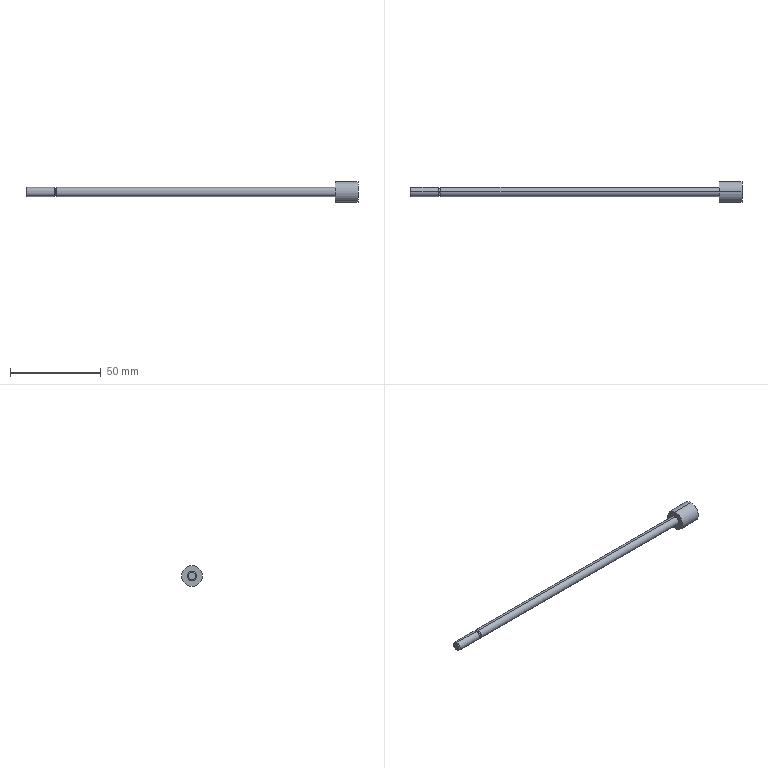Part | STEP file | 001-004-12PB125URod | 1 solid | 16 faces | box 182.85 x 11.5 x 11.5 mm | volume 4627 mm3 | cylinder 8 | cone 4 | plane 4 | commonest cylinder face diameters 5 x4 4.38 x2 11.5 x2
STEP:
#1=CARTESIAN_POINT('',(0.,0.,0.));
#2=DIRECTION('',(0.,0.,1.));
#3=DIRECTION('',(1.,0.,0.));
#4=AXIS2_PLACEMENT_3D('',#1,#2,#3);
#5=CARTESIAN_POINT('',(182.85,0.,5.75));
#6=VERTEX_POINT('',#5);
#7=CARTESIAN_POINT('',(182.85,0.,-5.75));
#8=VERTEX_POINT('',#7);
#9=CARTESIAN_POINT('',(182.85,0.,0.));
#10=DIRECTION('',(-1.,0.,0.));
#11=DIRECTION('',(0.,0.,1.));
#12=AXIS2_PLACEMENT_3D('',#9,#10,#11);
#13=CIRCLE('',#12,5.75);
#14=CARTESIAN_POINT('',(182.85,0.,0.));
#15=DIRECTION('',(-1.,0.,0.));
#16=DIRECTION('',(0.,0.,1.));
#17=AXIS2_PLACEMENT_3D('',#14,#15,#16);
#18=CYLINDRICAL_SURFACE('',#17,5.75);
#19=CARTESIAN_POINT('',(0.,0.));
#20=DIRECTION('',(1.,0.));
#21=VECTOR('',#20,1.);
#22=LINE('',#19,#21);
#23=(GEOMETRIC_REPRESENTATION_CONTEXT(2)PARAMETRIC_REPRESENTATION_CONTEXT()REPRESENTATION_CONTEXT('',''));
#24=DEFINITIONAL_REPRESENTATION('',(#22),#23);
#25=PCURVE('',#18,#24);
#26=CARTESIAN_POINT('',(182.85,5.75,0.));
#27=DIRECTION('',(-1.,0.,0.));
#28=DIRECTION('',(0.,0.,1.));
#29=AXIS2_PLACEMENT_3D('',#26,#27,#28);
#30=PLANE('',#29);
#31=CARTESIAN_POINT('',(0.,-5.75));
#32=DIRECTION('',(1.,0.));
#33=AXIS2_PLACEMENT_2D('',#31,#32);
#34=CIRCLE('',#33,5.75);
#35=(GEOMETRIC_REPRESENTATION_CONTEXT(2)PARAMETRIC_REPRESENTATION_CONTEXT()REPRESENTATION_CONTEXT('',''));
#36=DEFINITIONAL_REPRESENTATION('',(#34),#35);
#37=PCURVE('',#30,#36);
#38=SURFACE_CURVE('',#13,(#25,#37),.PCURVE_S1.);
#39=EDGE_CURVE('',#6,#8,#38,.T.);
#40=ORIENTED_EDGE('',*,*,#39,.T.);
#41=CARTESIAN_POINT('',(170.45,0.,-5.75));
#42=VERTEX_POINT('',#41);
#43=CARTESIAN_POINT('',(182.85,0.,-5.75));
#44=DIRECTION('',(-1.,0.,0.));
#45=VECTOR('',#44,1.);
#46=LINE('',#43,#45);
#47=CARTESIAN_POINT('',(3.142,0.));
#48=DIRECTION('',(0.,1.));
#49=VECTOR('',#48,1.);
#50=LINE('',#47,#49);
#51=(GEOMETRIC_REPRESENTATION_CONTEXT(2)PARAMETRIC_REPRESENTATION_CONTEXT()REPRESENTATION_CONTEXT('',''));
#52=DEFINITIONAL_REPRESENTATION('',(#50),#51);
#53=PCURVE('',#18,#52);
#54=CARTESIAN_POINT('',(182.85,0.,0.));
#55=DIRECTION('',(-1.,0.,0.));
#56=DIRECTION('',(0.,0.,1.));
#57=AXIS2_PLACEMENT_3D('',#54,#55,#56);
#58=CYLINDRICAL_SURFACE('',#57,5.75);
#59=CARTESIAN_POINT('',(3.142,0.));
#60=DIRECTION('',(0.,1.));
#61=VECTOR('',#60,1.);
#62=LINE('',#59,#61);
#63=(GEOMETRIC_REPRESENTATION_CONTEXT(2)PARAMETRIC_REPRESENTATION_CONTEXT()REPRESENTATION_CONTEXT('',''));
#64=DEFINITIONAL_REPRESENTATION('',(#62),#63);
#65=PCURVE('',#58,#64);
#66=SURFACE_CURVE('',#46,(#53,#65),.PCURVE_S1.);
#67=EDGE_CURVE('',#8,#42,#66,.T.);
#68=ORIENTED_EDGE('',*,*,#67,.T.);
#69=CARTESIAN_POINT('',(170.45,0.,5.75));
#70=VERTEX_POINT('',#69);
#71=CARTESIAN_POINT('',(170.45,0.,0.));
#72=DIRECTION('',(-1.,0.,0.));
#73=DIRECTION('',(0.,0.,1.));
#74=AXIS2_PLACEMENT_3D('',#71,#72,#73);
#75=CIRCLE('',#74,5.75);
#76=CARTESIAN_POINT('',(0.,12.4));
#77=DIRECTION('',(1.,0.));
#78=VECTOR('',#77,1.);
#79=LINE('',#76,#78);
#80=(GEOMETRIC_REPRESENTATION_CONTEXT(2)PARAMETRIC_REPRESENTATION_CONTEXT()REPRESENTATION_CONTEXT('',''));
#81=DEFINITIONAL_REPRESENTATION('',(#79),#80);
#82=PCURVE('',#18,#81);
#83=CARTESIAN_POINT('',(170.45,2.5,0.));
#84=DIRECTION('',(1.,0.,0.));
#85=DIRECTION('',(0.,0.,-1.));
#86=AXIS2_PLACEMENT_3D('',#83,#84,#85);
#87=PLANE('',#86);
#88=CARTESIAN_POINT('',(-5.75,-2.5));
#89=CARTESIAN_POINT('',(-5.75,7.459));
#90=CARTESIAN_POINT('',(2.875,2.48));
#91=CARTESIAN_POINT('',(11.5,-2.5));
#92=CARTESIAN_POINT('',(2.875,-7.48));
#93=CARTESIAN_POINT('',(-5.75,-12.459));
#94=CARTESIAN_POINT('',(-5.75,-2.5));
#95=(BOUNDED_CURVE()B_SPLINE_CURVE(2,(#88,#89,#90,#91,#92,#93,#94),.UNSPECIFIED.,.T.,.F.)B_SPLINE_CURVE_WITH_KNOTS((1,2,2,2,2,1),(-2.094,0.,2.094,4.189,6.283,8.378),.UNSPECIFIED.)CURVE()GEOMETRIC_REPRESENTATION_ITEM()RATIONAL_B_SPLINE_CURVE((1.,0.5,1.,0.5,1.,0.5,1.))REPRESENTATION_ITEM(''));
#96=(GEOMETRIC_REPRESENTATION_CONTEXT(2)PARAMETRIC_REPRESENTATION_CONTEXT()REPRESENTATION_CONTEXT('',''));
#97=DEFINITIONAL_REPRESENTATION('',(#95),#96);
#98=PCURVE('',#87,#97);
#99=SURFACE_CURVE('',#75,(#82,#98),.PCURVE_S1.);
#100=EDGE_CURVE('',#70,#42,#99,.T.);
#101=ORIENTED_EDGE('',*,*,#100,.F.);
#102=CARTESIAN_POINT('',(182.85,0.,5.75));
#103=DIRECTION('',(-1.,0.,0.));
#104=VECTOR('',#103,1.);
#105=LINE('',#102,#104);
#106=CARTESIAN_POINT('',(0.,0.));
#107=DIRECTION('',(0.,1.));
#108=VECTOR('',#107,1.);
#109=LINE('',#106,#108);
#110=(GEOMETRIC_REPRESENTATION_CONTEXT(2)PARAMETRIC_REPRESENTATION_CONTEXT()REPRESENTATION_CONTEXT('',''));
#111=DEFINITIONAL_REPRESENTATION('',(#109),#110);
#112=PCURVE('',#18,#111);
#113=CARTESIAN_POINT('',(6.283,0.));
#114=DIRECTION('',(0.,1.));
#115=VECTOR('',#114,1.);
#116=LINE('',#113,#115);
#117=(GEOMETRIC_REPRESENTATION_CONTEXT(2)PARAMETRIC_REPRESENTATION_CONTEXT()REPRESENTATION_CONTEXT('',''));
#118=DEFINITIONAL_REPRESENTATION('',(#116),#117);
#119=PCURVE('',#58,#118);
#120=SURFACE_CURVE('',#105,(#112,#119),.PCURVE_S1.);
#121=EDGE_CURVE('',#6,#70,#120,.T.);
#122=ORIENTED_EDGE('',*,*,#121,.F.);
#123=EDGE_LOOP('',(#40,#68,#101,#122));
#124=FACE_BOUND('',#123,.T.);
#125=ADVANCED_FACE('',(#124),#18,.T.);
#126=CARTESIAN_POINT('',(170.45,0.,2.5));
#127=VERTEX_POINT('',#126);
#128=CARTESIAN_POINT('',(170.45,0.,-2.5));
#129=VERTEX_POINT('',#128);
#130=CARTESIAN_POINT('',(170.45,0.,0.));
#131=DIRECTION('',(-1.,0.,0.));
#132=DIRECTION('',(0.,0.,1.));
#133=AXIS2_PLACEMENT_3D('',#130,#131,#132);
#134=CIRCLE('',#133,2.5);
#135=CARTESIAN_POINT('',(182.85,0.,0.));
#136=DIRECTION('',(-1.,0.,0.));
#137=DIRECTION('',(0.,0.,1.));
#138=AXIS2_PLACEMENT_3D('',#135,#136,#137);
#139=CYLINDRICAL_SURFACE('',#138,2.5);
#140=CARTESIAN_POINT('',(0.,12.4));
#141=DIRECTION('',(1.,0.));
#142=VECTOR('',#141,1.);
#143=LINE('',#140,#142);
#144=(GEOMETRIC_REPRESENTATION_CONTEXT(2)PARAMETRIC_REPRESENTATION_CONTEXT()REPRESENTATION_CONTEXT('',''));
#145=DEFINITIONAL_REPRESENTATION('',(#143),#144);
#146=PCURVE('',#139,#145);
#147=CARTESIAN_POINT('',(-2.5,-2.5));
#148=CARTESIAN_POINT('',(-2.5,1.83));
#149=CARTESIAN_POINT('',(1.25,-0.3349));
#150=CARTESIAN_POINT('',(5.,-2.5));
#151=CARTESIAN_POINT('',(1.25,-4.665));
#152=CARTESIAN_POINT('',(-2.5,-6.83));
#153=CARTESIAN_POINT('',(-2.5,-2.5));
#154=(BOUNDED_CURVE()B_SPLINE_CURVE(2,(#147,#148,#149,#150,#151,#152,#153),.UNSPECIFIED.,.T.,.F.)B_SPLINE_CURVE_WITH_KNOTS((1,2,2,2,2,1),(-2.094,0.,2.094,4.189,6.283,8.378),.UNSPECIFIED.)CURVE()GEOMETRIC_REPRESENTATION_ITEM()RATIONAL_B_SPLINE_CURVE((1.,0.5,1.,0.5,1.,0.5,1.))REPRESENTATION_ITEM(''));
#155=(GEOMETRIC_REPRESENTATION_CONTEXT(2)PARAMETRIC_REPRESENTATION_CONTEXT()REPRESENTATION_CONTEXT('',''));
#156=DEFINITIONAL_REPRESENTATION('',(#154),#155);
#157=PCURVE('',#87,#156);
#158=SURFACE_CURVE('',#134,(#146,#157),.PCURVE_S1.);
#159=EDGE_CURVE('',#127,#129,#158,.T.);
#160=ORIENTED_EDGE('',*,*,#159,.T.);
#161=CARTESIAN_POINT('',(17.,0.,-2.5));
#162=VERTEX_POINT('',#161);
#163=CARTESIAN_POINT('',(182.85,0.,-2.5));
#164=DIRECTION('',(-1.,0.,0.));
#165=VECTOR('',#164,1.);
#166=LINE('',#163,#165);
#167=CARTESIAN_POINT('',(3.142,0.));
#168=DIRECTION('',(0.,1.));
#169=VECTOR('',#168,1.);
#170=LINE('',#167,#169);
#171=(GEOMETRIC_REPRESENTATION_CONTEXT(2)PARAMETRIC_REPRESENTATION_CONTEXT()REPRESENTATION_CONTEXT('',''));
#172=DEFINITIONAL_REPRESENTATION('',(#170),#171);
#173=PCURVE('',#139,#172);
#174=CARTESIAN_POINT('',(182.85,0.,0.));
#175=DIRECTION('',(-1.,0.,0.));
#176=DIRECTION('',(0.,0.,1.));
#177=AXIS2_PLACEMENT_3D('',#174,#175,#176);
#178=CYLINDRICAL_SURFACE('',#177,2.5);
#179=CARTESIAN_POINT('',(3.142,0.));
#180=DIRECTION('',(0.,1.));
#181=VECTOR('',#180,1.);
#182=LINE('',#179,#181);
#183=(GEOMETRIC_REPRESENTATION_CONTEXT(2)PARAMETRIC_REPRESENTATION_CONTEXT()REPRESENTATION_CONTEXT('',''));
#184=DEFINITIONAL_REPRESENTATION('',(#182),#183);
#185=PCURVE('',#178,#184);
#186=SURFACE_CURVE('',#166,(#173,#185),.PCURVE_S1.);
#187=EDGE_CURVE('',#129,#162,#186,.T.);
#188=ORIENTED_EDGE('',*,*,#187,.T.);
#189=CARTESIAN_POINT('',(17.,0.,2.5));
#190=VERTEX_POINT('',#189);
#191=CARTESIAN_POINT('',(17.,0.,0.));
#192=DIRECTION('',(-1.,0.,0.));
#193=DIRECTION('',(0.,0.,1.));
#194=AXIS2_PLACEMENT_3D('',#191,#192,#193);
#195=CIRCLE('',#194,2.5);
#196=CARTESIAN_POINT('',(0.,165.85));
#197=DIRECTION('',(1.,0.));
#198=VECTOR('',#197,1.);
#199=LINE('',#196,#198);
#200=(GEOMETRIC_REPRESENTATION_CONTEXT(2)PARAMETRIC_REPRESENTATION_CONTEXT()REPRESENTATION_CONTEXT('',''));
#201=DEFINITIONAL_REPRESENTATION('',(#199),#200);
#202=PCURVE('',#139,#201);
#203=CARTESIAN_POINT('',(17.,0.,0.));
#204=DIRECTION('',(1.,0.,0.));
#205=DIRECTION('',(0.,0.,-1.));
#206=AXIS2_PLACEMENT_3D('',#203,#204,#205);
#207=CONICAL_SURFACE('',#206,2.5,0.555);
#208=CARTESIAN_POINT('',(3.142,0.));
#209=DIRECTION('',(-1.,0.));
#210=VECTOR('',#209,1.);
#211=LINE('',#208,#210);
#212=(GEOMETRIC_REPRESENTATION_CONTEXT(2)PARAMETRIC_REPRESENTATION_CONTEXT()REPRESENTATION_CONTEXT('',''));
#213=DEFINITIONAL_REPRESENTATION('',(#211),#212);
#214=PCURVE('',#207,#213);
#215=SURFACE_CURVE('',#195,(#202,#214),.PCURVE_S1.);
#216=EDGE_CURVE('',#190,#162,#215,.T.);
#217=ORIENTED_EDGE('',*,*,#216,.F.);
#218=CARTESIAN_POINT('',(182.85,0.,2.5));
#219=DIRECTION('',(-1.,0.,0.));
#220=VECTOR('',#219,1.);
#221=LINE('',#218,#220);
#222=CARTESIAN_POINT('',(0.,0.));
#223=DIRECTION('',(0.,1.));
#224=VECTOR('',#223,1.);
#225=LINE('',#222,#224);
#226=(GEOMETRIC_REPRESENTATION_CONTEXT(2)PARAMETRIC_REPRESENTATION_CONTEXT()REPRESENTATION_CONTEXT('',''));
#227=DEFINITIONAL_REPRESENTATION('',(#225),#226);
#228=PCURVE('',#139,#227);
#229=CARTESIAN_POINT('',(6.283,0.));
#230=DIRECTION('',(0.,1.));
#231=VECTOR('',#230,1.);
#232=LINE('',#229,#231);
#233=(GEOMETRIC_REPRESENTATION_CONTEXT(2)PARAMETRIC_REPRESENTATION_CONTEXT()REPRESENTATION_CONTEXT('',''));
#234=DEFINITIONAL_REPRESENTATION('',(#232),#233);
#235=PCURVE('',#178,#234);
#236=SURFACE_CURVE('',#221,(#228,#235),.PCURVE_S1.);
#237=EDGE_CURVE('',#127,#190,#236,.T.);
#238=ORIENTED_EDGE('',*,*,#237,.F.);
#239=EDGE_LOOP('',(#160,#188,#217,#238));
#240=FACE_BOUND('',#239,.T.);
#241=ADVANCED_FACE('',(#240),#139,.T.);
#242=CARTESIAN_POINT('',(16.5,0.,2.19));
#243=VERTEX_POINT('',#242);
#244=CARTESIAN_POINT('',(16.5,0.,-2.19));
#245=VERTEX_POINT('',#244);
#246=CARTESIAN_POINT('',(16.5,0.,0.));
#247=DIRECTION('',(-1.,0.,0.));
#248=DIRECTION('',(0.,0.,1.));
#249=AXIS2_PLACEMENT_3D('',#246,#247,#248);
#250=CIRCLE('',#249,2.19);
#251=CARTESIAN_POINT('',(3.142,-0.5));
#252=DIRECTION('',(-1.,0.));
#253=VECTOR('',#252,1.);
#254=LINE('',#251,#253);
#255=(GEOMETRIC_REPRESENTATION_CONTEXT(2)PARAMETRIC_REPRESENTATION_CONTEXT()REPRESENTATION_CONTEXT('',''));
#256=DEFINITIONAL_REPRESENTATION('',(#254),#255);
#257=PCURVE('',#207,#256);
#258=CARTESIAN_POINT('',(182.85,0.,0.));
#259=DIRECTION('',(-1.,0.,0.));
#260=DIRECTION('',(0.,0.,1.));
#261=AXIS2_PLACEMENT_3D('',#258,#259,#260);
#262=CYLINDRICAL_SURFACE('',#261,2.19);
#263=CARTESIAN_POINT('',(0.,166.35));
#264=DIRECTION('',(1.,0.));
#265=VECTOR('',#264,1.);
#266=LINE('',#263,#265);
#267=(GEOMETRIC_REPRESENTATION_CONTEXT(2)PARAMETRIC_REPRESENTATION_CONTEXT()REPRESENTATION_CONTEXT('',''));
#268=DEFINITIONAL_REPRESENTATION('',(#266),#267);
#269=PCURVE('',#262,#268);
#270=SURFACE_CURVE('',#250,(#257,#269),.PCURVE_S1.);
#271=EDGE_CURVE('',#243,#245,#270,.T.);
#272=ORIENTED_EDGE('',*,*,#271,.F.);
#273=CARTESIAN_POINT('',(17.,0.,2.5));
#274=DIRECTION('',(0.8499,0.,0.5269));
#275=VECTOR('',#274,1.);
#276=LINE('',#273,#275);
#277=CARTESIAN_POINT('',(3.142,0.));
#278=DIRECTION('',(0.,1.));
#279=VECTOR('',#278,1.);
#280=LINE('',#277,#279);
#281=(GEOMETRIC_REPRESENTATION_CONTEXT(2)PARAMETRIC_REPRESENTATION_CONTEXT()REPRESENTATION_CONTEXT('',''));
#282=DEFINITIONAL_REPRESENTATION('',(#280),#281);
#283=PCURVE('',#207,#282);
#284=CARTESIAN_POINT('',(17.,0.,0.));
#285=DIRECTION('',(1.,0.,0.));
#286=DIRECTION('',(0.,0.,-1.));
#287=AXIS2_PLACEMENT_3D('',#284,#285,#286);
#288=CONICAL_SURFACE('',#287,2.5,0.555);
#289=CARTESIAN_POINT('',(3.142,0.));
#290=DIRECTION('',(0.,1.));
#291=VECTOR('',#290,1.);
#292=LINE('',#289,#291);
#293=(GEOMETRIC_REPRESENTATION_CONTEXT(2)PARAMETRIC_REPRESENTATION_CONTEXT()REPRESENTATION_CONTEXT('',''));
#294=DEFINITIONAL_REPRESENTATION('',(#292),#293);
#295=PCURVE('',#288,#294);
#296=SURFACE_CURVE('',#276,(#283,#295),.PCURVE_S1.);
#297=EDGE_CURVE('',#243,#190,#296,.T.);
#298=ORIENTED_EDGE('',*,*,#297,.T.);
#299=ORIENTED_EDGE('',*,*,#216,.T.);
#300=CARTESIAN_POINT('',(17.,0.,-2.5));
#301=DIRECTION('',(0.8499,0.,-0.5269));
#302=VECTOR('',#301,1.);
#303=LINE('',#300,#302);
#304=CARTESIAN_POINT('',(0.,0.));
#305=DIRECTION('',(0.,1.));
#306=VECTOR('',#305,1.);
#307=LINE('',#304,#306);
#308=(GEOMETRIC_REPRESENTATION_CONTEXT(2)PARAMETRIC_REPRESENTATION_CONTEXT()REPRESENTATION_CONTEXT('',''));
#309=DEFINITIONAL_REPRESENTATION('',(#307),#308);
#310=PCURVE('',#207,#309);
#311=CARTESIAN_POINT('',(6.283,0.));
#312=DIRECTION('',(0.,1.));
#313=VECTOR('',#312,1.);
#314=LINE('',#311,#313);
#315=(GEOMETRIC_REPRESENTATION_CONTEXT(2)PARAMETRIC_REPRESENTATION_CONTEXT()REPRESENTATION_CONTEXT('',''));
#316=DEFINITIONAL_REPRESENTATION('',(#314),#315);
#317=PCURVE('',#288,#316);
#318=SURFACE_CURVE('',#303,(#310,#317),.PCURVE_S1.);
#319=EDGE_CURVE('',#245,#162,#318,.T.);
#320=ORIENTED_EDGE('',*,*,#319,.F.);
#321=EDGE_LOOP('',(#272,#298,#299,#320));
#322=FACE_BOUND('',#321,.T.);
#323=ADVANCED_FACE('',(#322),#207,.T.);
#324=ORIENTED_EDGE('',*,*,#271,.T.);
#325=CARTESIAN_POINT('',(15.5,0.,-2.19));
#326=VERTEX_POINT('',#325);
#327=CARTESIAN_POINT('',(182.85,0.,-2.19));
#328=DIRECTION('',(-1.,0.,0.));
#329=VECTOR('',#328,1.);
#330=LINE('',#327,#329);
#331=CARTESIAN_POINT('',(3.142,0.));
#332=DIRECTION('',(0.,1.));
#333=VECTOR('',#332,1.);
#334=LINE('',#331,#333);
#335=(GEOMETRIC_REPRESENTATION_CONTEXT(2)PARAMETRIC_REPRESENTATION_CONTEXT()REPRESENTATION_CONTEXT('',''));
#336=DEFINITIONAL_REPRESENTATION('',(#334),#335);
#337=PCURVE('',#262,#336);
#338=CARTESIAN_POINT('',(182.85,0.,0.));
#339=DIRECTION('',(-1.,0.,0.));
#340=DIRECTION('',(0.,0.,1.));
#341=AXIS2_PLACEMENT_3D('',#338,#339,#340);
#342=CYLINDRICAL_SURFACE('',#341,2.19);
#343=CARTESIAN_POINT('',(3.142,0.));
#344=DIRECTION('',(0.,1.));
#345=VECTOR('',#344,1.);
#346=LINE('',#343,#345);
#347=(GEOMETRIC_REPRESENTATION_CONTEXT(2)PARAMETRIC_REPRESENTATION_CONTEXT()REPRESENTATION_CONTEXT('',''));
#348=DEFINITIONAL_REPRESENTATION('',(#346),#347);
#349=PCURVE('',#342,#348);
#350=SURFACE_CURVE('',#330,(#337,#349),.PCURVE_S1.);
#351=EDGE_CURVE('',#245,#326,#350,.T.);
#352=ORIENTED_EDGE('',*,*,#351,.T.);
#353=CARTESIAN_POINT('',(15.5,0.,2.19));
#354=VERTEX_POINT('',#353);
#355=CARTESIAN_POINT('',(15.5,0.,0.));
#356=DIRECTION('',(-1.,0.,0.));
#357=DIRECTION('',(0.,0.,1.));
#358=AXIS2_PLACEMENT_3D('',#355,#356,#357);
#359=CIRCLE('',#358,2.19);
#360=CARTESIAN_POINT('',(0.,167.35));
#361=DIRECTION('',(1.,0.));
#362=VECTOR('',#361,1.);
#363=LINE('',#360,#362);
#364=(GEOMETRIC_REPRESENTATION_CONTEXT(2)PARAMETRIC_REPRESENTATION_CONTEXT()REPRESENTATION_CONTEXT('',''));
#365=DEFINITIONAL_REPRESENTATION('',(#363),#364);
#366=PCURVE('',#262,#365);
#367=CARTESIAN_POINT('',(15.5,2.5,0.));
#368=DIRECTION('',(-1.,0.,0.));
#369=DIRECTION('',(0.,0.,1.));
#370=AXIS2_PLACEMENT_3D('',#367,#368,#369);
#371=PLANE('',#370);
#372=CARTESIAN_POINT('',(0.,-2.5));
#373=DIRECTION('',(1.,0.));
#374=AXIS2_PLACEMENT_2D('',#372,#373);
#375=CIRCLE('',#374,2.19);
#376=(GEOMETRIC_REPRESENTATION_CONTEXT(2)PARAMETRIC_REPRESENTATION_CONTEXT()REPRESENTATION_CONTEXT('',''));
#377=DEFINITIONAL_REPRESENTATION('',(#375),#376);
#378=PCURVE('',#371,#377);
#379=SURFACE_CURVE('',#359,(#366,#378),.PCURVE_S1.);
#380=EDGE_CURVE('',#354,#326,#379,.T.);
#381=ORIENTED_EDGE('',*,*,#380,.F.);
#382=CARTESIAN_POINT('',(182.85,0.,2.19));
#383=DIRECTION('',(-1.,0.,0.));
#384=VECTOR('',#383,1.);
#385=LINE('',#382,#384);
#386=CARTESIAN_POINT('',(0.,0.));
#387=DIRECTION('',(0.,1.));
#388=VECTOR('',#387,1.);
#389=LINE('',#386,#388);
#390=(GEOMETRIC_REPRESENTATION_CONTEXT(2)PARAMETRIC_REPRESENTATION_CONTEXT()REPRESENTATION_CONTEXT('',''));
#391=DEFINITIONAL_REPRESENTATION('',(#389),#390);
#392=PCURVE('',#262,#391);
#393=CARTESIAN_POINT('',(6.283,0.));
#394=DIRECTION('',(0.,1.));
#395=VECTOR('',#394,1.);
#396=LINE('',#393,#395);
#397=(GEOMETRIC_REPRESENTATION_CONTEXT(2)PARAMETRIC_REPRESENTATION_CONTEXT()REPRESENTATION_CONTEXT('',''));
#398=DEFINITIONAL_REPRESENTATION('',(#396),#397);
#399=PCURVE('',#342,#398);
#400=SURFACE_CURVE('',#385,(#392,#399),.PCURVE_S1.);
#401=EDGE_CURVE('',#243,#354,#400,.T.);
#402=ORIENTED_EDGE('',*,*,#401,.F.);
#403=EDGE_LOOP('',(#324,#352,#381,#402));
#404=FACE_BOUND('',#403,.T.);
#405=ADVANCED_FACE('',(#404),#262,.T.);
#406=CARTESIAN_POINT('',(15.5,0.,2.5));
#407=VERTEX_POINT('',#406);
#408=CARTESIAN_POINT('',(15.5,0.,-2.5));
#409=VERTEX_POINT('',#408);
#410=CARTESIAN_POINT('',(15.5,0.,0.));
#411=DIRECTION('',(-1.,0.,0.));
#412=DIRECTION('',(0.,0.,1.));
#413=AXIS2_PLACEMENT_3D('',#410,#411,#412);
#414=CIRCLE('',#413,2.5);
#415=CARTESIAN_POINT('',(182.85,0.,0.));
#416=DIRECTION('',(-1.,0.,0.));
#417=DIRECTION('',(0.,0.,1.));
#418=AXIS2_PLACEMENT_3D('',#415,#416,#417);
#419=CYLINDRICAL_SURFACE('',#418,2.5);
#420=CARTESIAN_POINT('',(0.,167.35));
#421=DIRECTION('',(1.,0.));
#422=VECTOR('',#421,1.);
#423=LINE('',#420,#422);
#424=(GEOMETRIC_REPRESENTATION_CONTEXT(2)PARAMETRIC_REPRESENTATION_CONTEXT()REPRESENTATION_CONTEXT('',''));
#425=DEFINITIONAL_REPRESENTATION('',(#423),#424);
#426=PCURVE('',#419,#425);
#427=CARTESIAN_POINT('',(0.,-2.5));
#428=DIRECTION('',(1.,0.));
#429=AXIS2_PLACEMENT_2D('',#427,#428);
#430=CIRCLE('',#429,2.5);
#431=(GEOMETRIC_REPRESENTATION_CONTEXT(2)PARAMETRIC_REPRESENTATION_CONTEXT()REPRESENTATION_CONTEXT('',''));
#432=DEFINITIONAL_REPRESENTATION('',(#430),#431);
#433=PCURVE('',#371,#432);
#434=SURFACE_CURVE('',#414,(#426,#433),.PCURVE_S1.);
#435=EDGE_CURVE('',#407,#409,#434,.T.);
#436=ORIENTED_EDGE('',*,*,#435,.T.);
#437=CARTESIAN_POINT('',(0.4905,0.,-2.5));
#438=VERTEX_POINT('',#437);
#439=CARTESIAN_POINT('',(182.85,0.,-2.5));
#440=DIRECTION('',(-1.,0.,0.));
#441=VECTOR('',#440,1.);
#442=LINE('',#439,#441);
#443=CARTESIAN_POINT('',(3.142,0.));
#444=DIRECTION('',(0.,1.));
#445=VECTOR('',#444,1.);
#446=LINE('',#443,#445);
#447=(GEOMETRIC_REPRESENTATION_CONTEXT(2)PARAMETRIC_REPRESENTATION_CONTEXT()REPRESENTATION_CONTEXT('',''));
#448=DEFINITIONAL_REPRESENTATION('',(#446),#447);
#449=PCURVE('',#419,#448);
#450=CARTESIAN_POINT('',(182.85,0.,0.));
#451=DIRECTION('',(-1.,0.,0.));
#452=DIRECTION('',(0.,0.,1.));
#453=AXIS2_PLACEMENT_3D('',#450,#451,#452);
#454=CYLINDRICAL_SURFACE('',#453,2.5);
#455=CARTESIAN_POINT('',(3.142,0.));
#456=DIRECTION('',(0.,1.));
#457=VECTOR('',#456,1.);
#458=LINE('',#455,#457);
#459=(GEOMETRIC_REPRESENTATION_CONTEXT(2)PARAMETRIC_REPRESENTATION_CONTEXT()REPRESENTATION_CONTEXT('',''));
#460=DEFINITIONAL_REPRESENTATION('',(#458),#459);
#461=PCURVE('',#454,#460);
#462=SURFACE_CURVE('',#442,(#449,#461),.PCURVE_S1.);
#463=EDGE_CURVE('',#409,#438,#462,.T.);
#464=ORIENTED_EDGE('',*,*,#463,.T.);
#465=CARTESIAN_POINT('',(0.4905,0.,2.5));
#466=VERTEX_POINT('',#465);
#467=CARTESIAN_POINT('',(0.4905,0.,0.));
#468=DIRECTION('',(-1.,0.,0.));
#469=DIRECTION('',(0.,0.,1.));
#470=AXIS2_PLACEMENT_3D('',#467,#468,#469);
#471=CIRCLE('',#470,2.5);
#472=CARTESIAN_POINT('',(0.,182.359));
#473=DIRECTION('',(1.,0.));
#474=VECTOR('',#473,1.);
#475=LINE('',#472,#474);
#476=(GEOMETRIC_REPRESENTATION_CONTEXT(2)PARAMETRIC_REPRESENTATION_CONTEXT()REPRESENTATION_CONTEXT('',''));
#477=DEFINITIONAL_REPRESENTATION('',(#475),#476);
#478=PCURVE('',#419,#477);
#479=CARTESIAN_POINT('',(0.4905,0.,0.));
#480=DIRECTION('',(1.,0.,0.));
#481=DIRECTION('',(0.,0.,-1.));
#482=AXIS2_PLACEMENT_3D('',#479,#480,#481);
#483=CONICAL_SURFACE('',#482,2.5,0.7854);
#484=CARTESIAN_POINT('',(3.142,0.));
#485=DIRECTION('',(-1.,0.));
#486=VECTOR('',#485,1.);
#487=LINE('',#484,#486);
#488=(GEOMETRIC_REPRESENTATION_CONTEXT(2)PARAMETRIC_REPRESENTATION_CONTEXT()REPRESENTATION_CONTEXT('',''));
#489=DEFINITIONAL_REPRESENTATION('',(#487),#488);
#490=PCURVE('',#483,#489);
#491=SURFACE_CURVE('',#471,(#478,#490),.PCURVE_S1.);
#492=EDGE_CURVE('',#466,#438,#491,.T.);
#493=ORIENTED_EDGE('',*,*,#492,.F.);
#494=CARTESIAN_POINT('',(182.85,0.,2.5));
#495=DIRECTION('',(-1.,0.,0.));
#496=VECTOR('',#495,1.);
#497=LINE('',#494,#496);
#498=CARTESIAN_POINT('',(0.,0.));
#499=DIRECTION('',(0.,1.));
#500=VECTOR('',#499,1.);
#501=LINE('',#498,#500);
#502=(GEOMETRIC_REPRESENTATION_CONTEXT(2)PARAMETRIC_REPRESENTATION_CONTEXT()REPRESENTATION_CONTEXT('',''));
#503=DEFINITIONAL_REPRESENTATION('',(#501),#502);
#504=PCURVE('',#419,#503);
#505=CARTESIAN_POINT('',(6.283,0.));
#506=DIRECTION('',(0.,1.));
#507=VECTOR('',#506,1.);
#508=LINE('',#505,#507);
#509=(GEOMETRIC_REPRESENTATION_CONTEXT(2)PARAMETRIC_REPRESENTATION_CONTEXT()REPRESENTATION_CONTEXT('',''));
#510=DEFINITIONAL_REPRESENTATION('',(#508),#509);
#511=PCURVE('',#454,#510);
#512=SURFACE_CURVE('',#497,(#504,#511),.PCURVE_S1.);
#513=EDGE_CURVE('',#407,#466,#512,.T.);
#514=ORIENTED_EDGE('',*,*,#513,.F.);
#515=EDGE_LOOP('',(#436,#464,#493,#514));
#516=FACE_BOUND('',#515,.T.);
#517=ADVANCED_FACE('',(#516),#419,.T.);
#518=CARTESIAN_POINT('',(0.,0.,2.01));
#519=VERTEX_POINT('',#518);
#520=CARTESIAN_POINT('',(0.,0.,-2.01));
#521=VERTEX_POINT('',#520);
#522=CARTESIAN_POINT('',(0.,0.,0.));
#523=DIRECTION('',(-1.,0.,0.));
#524=DIRECTION('',(0.,0.,1.));
#525=AXIS2_PLACEMENT_3D('',#522,#523,#524);
#526=CIRCLE('',#525,2.01);
#527=CARTESIAN_POINT('',(3.142,-0.4905));
#528=DIRECTION('',(-1.,0.));
#529=VECTOR('',#528,1.);
#530=LINE('',#527,#529);
#531=(GEOMETRIC_REPRESENTATION_CONTEXT(2)PARAMETRIC_REPRESENTATION_CONTEXT()REPRESENTATION_CONTEXT('',''));
#532=DEFINITIONAL_REPRESENTATION('',(#530),#531);
#533=PCURVE('',#483,#532);
#534=CARTESIAN_POINT('',(0.,0.,0.));
#535=DIRECTION('',(1.,0.,0.));
#536=DIRECTION('',(0.,0.,-1.));
#537=AXIS2_PLACEMENT_3D('',#534,#535,#536);
#538=PLANE('',#537);
#539=CARTESIAN_POINT('',(-2.01,0.));
#540=CARTESIAN_POINT('',(-2.01,3.481));
#541=CARTESIAN_POINT('',(1.005,1.74));
#542=CARTESIAN_POINT('',(4.019,0.));
#543=CARTESIAN_POINT('',(1.005,-1.74));
#544=CARTESIAN_POINT('',(-2.01,-3.481));
#545=CARTESIAN_POINT('',(-2.01,0.));
#546=(BOUNDED_CURVE()B_SPLINE_CURVE(2,(#539,#540,#541,#542,#543,#544,#545),.UNSPECIFIED.,.T.,.F.)B_SPLINE_CURVE_WITH_KNOTS((1,2,2,2,2,1),(-2.094,0.,2.094,4.189,6.283,8.378),.UNSPECIFIED.)CURVE()GEOMETRIC_REPRESENTATION_ITEM()RATIONAL_B_SPLINE_CURVE((1.,0.5,1.,0.5,1.,0.5,1.))REPRESENTATION_ITEM(''));
#547=(GEOMETRIC_REPRESENTATION_CONTEXT(2)PARAMETRIC_REPRESENTATION_CONTEXT()REPRESENTATION_CONTEXT('',''));
#548=DEFINITIONAL_REPRESENTATION('',(#546),#547);
#549=PCURVE('',#538,#548);
#550=SURFACE_CURVE('',#526,(#533,#549),.PCURVE_S1.);
#551=EDGE_CURVE('',#519,#521,#550,.T.);
#552=ORIENTED_EDGE('',*,*,#551,.F.);
#553=CARTESIAN_POINT('',(0.4905,0.,2.5));
#554=DIRECTION('',(0.7071,0.,0.7071));
#555=VECTOR('',#554,1.);
#556=LINE('',#553,#555);
#557=CARTESIAN_POINT('',(3.142,0.));
#558=DIRECTION('',(0.,1.));
#559=VECTOR('',#558,1.);
#560=LINE('',#557,#559);
#561=(GEOMETRIC_REPRESENTATION_CONTEXT(2)PARAMETRIC_REPRESENTATION_CONTEXT()REPRESENTATION_CONTEXT('',''));
#562=DEFINITIONAL_REPRESENTATION('',(#560),#561);
#563=PCURVE('',#483,#562);
#564=CARTESIAN_POINT('',(0.4905,0.,0.));
#565=DIRECTION('',(1.,0.,0.));
#566=DIRECTION('',(0.,0.,-1.));
#567=AXIS2_PLACEMENT_3D('',#564,#565,#566);
#568=CONICAL_SURFACE('',#567,2.5,0.7854);
#569=CARTESIAN_POINT('',(3.142,0.));
#570=DIRECTION('',(0.,1.));
#571=VECTOR('',#570,1.);
#572=LINE('',#569,#571);
#573=(GEOMETRIC_REPRESENTATION_CONTEXT(2)PARAMETRIC_REPRESENTATION_CONTEXT()REPRESENTATION_CONTEXT('',''));
#574=DEFINITIONAL_REPRESENTATION('',(#572),#573);
#575=PCURVE('',#568,#574);
#576=SURFACE_CURVE('',#556,(#563,#575),.PCURVE_S1.);
#577=EDGE_CURVE('',#519,#466,#576,.T.);
#578=ORIENTED_EDGE('',*,*,#577,.T.);
#579=ORIENTED_EDGE('',*,*,#492,.T.);
#580=CARTESIAN_POINT('',(0.4905,0.,-2.5));
#581=DIRECTION('',(0.7071,0.,-0.7071));
#582=VECTOR('',#581,1.);
#583=LINE('',#580,#582);
#584=CARTESIAN_POINT('',(0.,0.));
#585=DIRECTION('',(0.,1.));
#586=VECTOR('',#585,1.);
#587=LINE('',#584,#586);
#588=(GEOMETRIC_REPRESENTATION_CONTEXT(2)PARAMETRIC_REPRESENTATION_CONTEXT()REPRESENTATION_CONTEXT('',''));
#589=DEFINITIONAL_REPRESENTATION('',(#587),#588);
#590=PCURVE('',#483,#589);
#591=CARTESIAN_POINT('',(6.283,0.));
#592=DIRECTION('',(0.,1.));
#593=VECTOR('',#592,1.);
#594=LINE('',#591,#593);
#595=(GEOMETRIC_REPRESENTATION_CONTEXT(2)PARAMETRIC_REPRESENTATION_CONTEXT()REPRESENTATION_CONTEXT('',''));
#596=DEFINITIONAL_REPRESENTATION('',(#594),#595);
#597=PCURVE('',#568,#596);
#598=SURFACE_CURVE('',#583,(#590,#597),.PCURVE_S1.);
#599=EDGE_CURVE('',#521,#438,#598,.T.);
#600=ORIENTED_EDGE('',*,*,#599,.F.);
#601=EDGE_LOOP('',(#552,#578,#579,#600));
#602=FACE_BOUND('',#601,.T.);
#603=ADVANCED_FACE('',(#602),#483,.T.);
#604=CARTESIAN_POINT('',(0.,0.,0.));
#605=DIRECTION('',(-1.,0.,0.));
#606=DIRECTION('',(0.,0.,1.));
#607=AXIS2_PLACEMENT_3D('',#604,#605,#606);
#608=CIRCLE('',#607,2.01);
#609=CARTESIAN_POINT('',(-2.01,0.));
#610=CARTESIAN_POINT('',(-2.01,3.481));
#611=CARTESIAN_POINT('',(1.005,1.74));
#612=CARTESIAN_POINT('',(4.019,0.));
#613=CARTESIAN_POINT('',(1.005,-1.74));
#614=CARTESIAN_POINT('',(-2.01,-3.481));
#615=CARTESIAN_POINT('',(-2.01,0.));
#616=(BOUNDED_CURVE()B_SPLINE_CURVE(2,(#609,#610,#611,#612,#613,#614,#615),.UNSPECIFIED.,.T.,.F.)B_SPLINE_CURVE_WITH_KNOTS((1,2,2,2,2,1),(-2.094,0.,2.094,4.189,6.283,8.378),.UNSPECIFIED.)CURVE()GEOMETRIC_REPRESENTATION_ITEM()RATIONAL_B_SPLINE_CURVE((1.,0.5,1.,0.5,1.,0.5,1.))REPRESENTATION_ITEM(''));
#617=(GEOMETRIC_REPRESENTATION_CONTEXT(2)PARAMETRIC_REPRESENTATION_CONTEXT()REPRESENTATION_CONTEXT('',''));
#618=DEFINITIONAL_REPRESENTATION('',(#616),#617);
#619=PCURVE('',#538,#618);
#620=CARTESIAN_POINT('',(9.425,-0.4905));
#621=DIRECTION('',(-1.,0.));
#622=VECTOR('',#621,1.);
#623=LINE('',#620,#622);
#624=(GEOMETRIC_REPRESENTATION_CONTEXT(2)PARAMETRIC_REPRESENTATION_CONTEXT()REPRESENTATION_CONTEXT('',''));
#625=DEFINITIONAL_REPRESENTATION('',(#623),#624);
#626=PCURVE('',#568,#625);
#627=SURFACE_CURVE('',#608,(#619,#626),.PCURVE_S1.);
#628=EDGE_CURVE('',#521,#519,#627,.T.);
#629=ORIENTED_EDGE('',*,*,#628,.T.);
#630=ORIENTED_EDGE('',*,*,#551,.T.);
#631=EDGE_LOOP('',(#629,#630));
#632=FACE_BOUND('',#631,.T.);
#633=ADVANCED_FACE('',(#632),#538,.F.);
#634=ORIENTED_EDGE('',*,*,#577,.F.);
#635=ORIENTED_EDGE('',*,*,#628,.F.);
#636=ORIENTED_EDGE('',*,*,#599,.T.);
#637=CARTESIAN_POINT('',(0.4905,0.,0.));
#638=DIRECTION('',(-1.,0.,0.));
#639=DIRECTION('',(0.,0.,1.));
#640=AXIS2_PLACEMENT_3D('',#637,#638,#639);
#641=CIRCLE('',#640,2.5);
#642=CARTESIAN_POINT('',(9.425,0.));
#643=DIRECTION('',(-1.,0.));
#644=VECTOR('',#643,1.);
#645=LINE('',#642,#644);
#646=(GEOMETRIC_REPRESENTATION_CONTEXT(2)PARAMETRIC_REPRESENTATION_CONTEXT()REPRESENTATION_CONTEXT('',''));
#647=DEFINITIONAL_REPRESENTATION('',(#645),#646);
#648=PCURVE('',#568,#647);
#649=CARTESIAN_POINT('',(0.,182.359));
#650=DIRECTION('',(1.,0.));
#651=VECTOR('',#650,1.);
#652=LINE('',#649,#651);
#653=(GEOMETRIC_REPRESENTATION_CONTEXT(2)PARAMETRIC_REPRESENTATION_CONTEXT()REPRESENTATION_CONTEXT('',''));
#654=DEFINITIONAL_REPRESENTATION('',(#652),#653);
#655=PCURVE('',#454,#654);
#656=SURFACE_CURVE('',#641,(#648,#655),.PCURVE_S1.);
#657=EDGE_CURVE('',#438,#466,#656,.T.);
#658=ORIENTED_EDGE('',*,*,#657,.T.);
#659=EDGE_LOOP('',(#634,#635,#636,#658));
#660=FACE_BOUND('',#659,.T.);
#661=ADVANCED_FACE('',(#660),#568,.T.);
#662=ORIENTED_EDGE('',*,*,#463,.F.);
#663=CARTESIAN_POINT('',(15.5,0.,0.));
#664=DIRECTION('',(-1.,0.,0.));
#665=DIRECTION('',(0.,0.,1.));
#666=AXIS2_PLACEMENT_3D('',#663,#664,#665);
#667=CIRCLE('',#666,2.5);
#668=CARTESIAN_POINT('',(0.,167.35));
#669=DIRECTION('',(1.,0.));
#670=VECTOR('',#669,1.);
#671=LINE('',#668,#670);
#672=(GEOMETRIC_REPRESENTATION_CONTEXT(2)PARAMETRIC_REPRESENTATION_CONTEXT()REPRESENTATION_CONTEXT('',''));
#673=DEFINITIONAL_REPRESENTATION('',(#671),#672);
#674=PCURVE('',#454,#673);
#675=CARTESIAN_POINT('',(0.,-2.5));
#676=DIRECTION('',(1.,0.));
#677=AXIS2_PLACEMENT_2D('',#675,#676);
#678=CIRCLE('',#677,2.5);
#679=(GEOMETRIC_REPRESENTATION_CONTEXT(2)PARAMETRIC_REPRESENTATION_CONTEXT()REPRESENTATION_CONTEXT('',''));
#680=DEFINITIONAL_REPRESENTATION('',(#678),#679);
#681=PCURVE('',#371,#680);
#682=SURFACE_CURVE('',#667,(#674,#681),.PCURVE_S1.);
#683=EDGE_CURVE('',#409,#407,#682,.T.);
#684=ORIENTED_EDGE('',*,*,#683,.T.);
#685=ORIENTED_EDGE('',*,*,#513,.T.);
#686=ORIENTED_EDGE('',*,*,#657,.F.);
#687=EDGE_LOOP('',(#662,#684,#685,#686));
#688=FACE_BOUND('',#687,.T.);
#689=ADVANCED_FACE('',(#688),#454,.T.);
#690=ORIENTED_EDGE('',*,*,#435,.F.);
#691=ORIENTED_EDGE('',*,*,#683,.F.);
#692=EDGE_LOOP('',(#690,#691));
#693=FACE_BOUND('',#692,.T.);
#694=ORIENTED_EDGE('',*,*,#380,.T.);
#695=CARTESIAN_POINT('',(15.5,0.,0.));
#696=DIRECTION('',(-1.,0.,0.));
#697=DIRECTION('',(0.,0.,1.));
#698=AXIS2_PLACEMENT_3D('',#695,#696,#697);
#699=CIRCLE('',#698,2.19);
#700=CARTESIAN_POINT('',(0.,-2.5));
#701=DIRECTION('',(1.,0.));
#702=AXIS2_PLACEMENT_2D('',#700,#701);
#703=CIRCLE('',#702,2.19);
#704=(GEOMETRIC_REPRESENTATION_CONTEXT(2)PARAMETRIC_REPRESENTATION_CONTEXT()REPRESENTATION_CONTEXT('',''));
#705=DEFINITIONAL_REPRESENTATION('',(#703),#704);
#706=PCURVE('',#371,#705);
#707=CARTESIAN_POINT('',(0.,167.35));
#708=DIRECTION('',(1.,0.));
#709=VECTOR('',#708,1.);
#710=LINE('',#707,#709);
#711=(GEOMETRIC_REPRESENTATION_CONTEXT(2)PARAMETRIC_REPRESENTATION_CONTEXT()REPRESENTATION_CONTEXT('',''));
#712=DEFINITIONAL_REPRESENTATION('',(#710),#711);
#713=PCURVE('',#342,#712);
#714=SURFACE_CURVE('',#699,(#706,#713),.PCURVE_S1.);
#715=EDGE_CURVE('',#326,#354,#714,.T.);
#716=ORIENTED_EDGE('',*,*,#715,.T.);
#717=EDGE_LOOP('',(#694,#716));
#718=FACE_BOUND('',#717,.T.);
#719=ADVANCED_FACE('',(#693,#718),#371,.F.);
#720=ORIENTED_EDGE('',*,*,#351,.F.);
#721=CARTESIAN_POINT('',(16.5,0.,0.));
#722=DIRECTION('',(-1.,0.,0.));
#723=DIRECTION('',(0.,0.,1.));
#724=AXIS2_PLACEMENT_3D('',#721,#722,#723);
#725=CIRCLE('',#724,2.19);
#726=CARTESIAN_POINT('',(0.,166.35));
#727=DIRECTION('',(1.,0.));
#728=VECTOR('',#727,1.);
#729=LINE('',#726,#728);
#730=(GEOMETRIC_REPRESENTATION_CONTEXT(2)PARAMETRIC_REPRESENTATION_CONTEXT()REPRESENTATION_CONTEXT('',''));
#731=DEFINITIONAL_REPRESENTATION('',(#729),#730);
#732=PCURVE('',#342,#731);
#733=CARTESIAN_POINT('',(9.425,-0.5));
#734=DIRECTION('',(-1.,0.));
#735=VECTOR('',#734,1.);
#736=LINE('',#733,#735);
#737=(GEOMETRIC_REPRESENTATION_CONTEXT(2)PARAMETRIC_REPRESENTATION_CONTEXT()REPRESENTATION_CONTEXT('',''));
#738=DEFINITIONAL_REPRESENTATION('',(#736),#737);
#739=PCURVE('',#288,#738);
#740=SURFACE_CURVE('',#725,(#732,#739),.PCURVE_S1.);
#741=EDGE_CURVE('',#245,#243,#740,.T.);
#742=ORIENTED_EDGE('',*,*,#741,.T.);
#743=ORIENTED_EDGE('',*,*,#401,.T.);
#744=ORIENTED_EDGE('',*,*,#715,.F.);
#745=EDGE_LOOP('',(#720,#742,#743,#744));
#746=FACE_BOUND('',#745,.T.);
#747=ADVANCED_FACE('',(#746),#342,.T.);
#748=ORIENTED_EDGE('',*,*,#297,.F.);
#749=ORIENTED_EDGE('',*,*,#741,.F.);
#750=ORIENTED_EDGE('',*,*,#319,.T.);
#751=CARTESIAN_POINT('',(17.,0.,0.));
#752=DIRECTION('',(-1.,0.,0.));
#753=DIRECTION('',(0.,0.,1.));
#754=AXIS2_PLACEMENT_3D('',#751,#752,#753);
#755=CIRCLE('',#754,2.5);
#756=CARTESIAN_POINT('',(9.425,0.));
#757=DIRECTION('',(-1.,0.));
#758=VECTOR('',#757,1.);
#759=LINE('',#756,#758);
#760=(GEOMETRIC_REPRESENTATION_CONTEXT(2)PARAMETRIC_REPRESENTATION_CONTEXT()REPRESENTATION_CONTEXT('',''));
#761=DEFINITIONAL_REPRESENTATION('',(#759),#760);
#762=PCURVE('',#288,#761);
#763=CARTESIAN_POINT('',(0.,165.85));
#764=DIRECTION('',(1.,0.));
#765=VECTOR('',#764,1.);
#766=LINE('',#763,#765);
#767=(GEOMETRIC_REPRESENTATION_CONTEXT(2)PARAMETRIC_REPRESENTATION_CONTEXT()REPRESENTATION_CONTEXT('',''));
#768=DEFINITIONAL_REPRESENTATION('',(#766),#767);
#769=PCURVE('',#178,#768);
#770=SURFACE_CURVE('',#755,(#762,#769),.PCURVE_S1.);
#771=EDGE_CURVE('',#162,#190,#770,.T.);
#772=ORIENTED_EDGE('',*,*,#771,.T.);
#773=EDGE_LOOP('',(#748,#749,#750,#772));
#774=FACE_BOUND('',#773,.T.);
#775=ADVANCED_FACE('',(#774),#288,.T.);
#776=ORIENTED_EDGE('',*,*,#187,.F.);
#777=CARTESIAN_POINT('',(170.45,0.,0.));
#778=DIRECTION('',(-1.,0.,0.));
#779=DIRECTION('',(0.,0.,1.));
#780=AXIS2_PLACEMENT_3D('',#777,#778,#779);
#781=CIRCLE('',#780,2.5);
#782=CARTESIAN_POINT('',(0.,12.4));
#783=DIRECTION('',(1.,0.));
#784=VECTOR('',#783,1.);
#785=LINE('',#782,#784);
#786=(GEOMETRIC_REPRESENTATION_CONTEXT(2)PARAMETRIC_REPRESENTATION_CONTEXT()REPRESENTATION_CONTEXT('',''));
#787=DEFINITIONAL_REPRESENTATION('',(#785),#786);
#788=PCURVE('',#178,#787);
#789=CARTESIAN_POINT('',(-2.5,-2.5));
#790=CARTESIAN_POINT('',(-2.5,1.83));
#791=CARTESIAN_POINT('',(1.25,-0.3349));
#792=CARTESIAN_POINT('',(5.,-2.5));
#793=CARTESIAN_POINT('',(1.25,-4.665));
#794=CARTESIAN_POINT('',(-2.5,-6.83));
#795=CARTESIAN_POINT('',(-2.5,-2.5));
#796=(BOUNDED_CURVE()B_SPLINE_CURVE(2,(#789,#790,#791,#792,#793,#794,#795),.UNSPECIFIED.,.T.,.F.)B_SPLINE_CURVE_WITH_KNOTS((1,2,2,2,2,1),(-2.094,0.,2.094,4.189,6.283,8.378),.UNSPECIFIED.)CURVE()GEOMETRIC_REPRESENTATION_ITEM()RATIONAL_B_SPLINE_CURVE((1.,0.5,1.,0.5,1.,0.5,1.))REPRESENTATION_ITEM(''));
#797=(GEOMETRIC_REPRESENTATION_CONTEXT(2)PARAMETRIC_REPRESENTATION_CONTEXT()REPRESENTATION_CONTEXT('',''));
#798=DEFINITIONAL_REPRESENTATION('',(#796),#797);
#799=PCURVE('',#87,#798);
#800=SURFACE_CURVE('',#781,(#788,#799),.PCURVE_S1.);
#801=EDGE_CURVE('',#129,#127,#800,.T.);
#802=ORIENTED_EDGE('',*,*,#801,.T.);
#803=ORIENTED_EDGE('',*,*,#237,.T.);
#804=ORIENTED_EDGE('',*,*,#771,.F.);
#805=EDGE_LOOP('',(#776,#802,#803,#804));
#806=FACE_BOUND('',#805,.T.);
#807=ADVANCED_FACE('',(#806),#178,.T.);
#808=ORIENTED_EDGE('',*,*,#159,.F.);
#809=ORIENTED_EDGE('',*,*,#801,.F.);
#810=EDGE_LOOP('',(#808,#809));
#811=FACE_BOUND('',#810,.T.);
#812=ORIENTED_EDGE('',*,*,#100,.T.);
#813=CARTESIAN_POINT('',(170.45,0.,0.));
#814=DIRECTION('',(-1.,0.,0.));
#815=DIRECTION('',(0.,0.,1.));
#816=AXIS2_PLACEMENT_3D('',#813,#814,#815);
#817=CIRCLE('',#816,5.75);
#818=CARTESIAN_POINT('',(-5.75,-2.5));
#819=CARTESIAN_POINT('',(-5.75,7.459));
#820=CARTESIAN_POINT('',(2.875,2.48));
#821=CARTESIAN_POINT('',(11.5,-2.5));
#822=CARTESIAN_POINT('',(2.875,-7.48));
#823=CARTESIAN_POINT('',(-5.75,-12.459));
#824=CARTESIAN_POINT('',(-5.75,-2.5));
#825=(BOUNDED_CURVE()B_SPLINE_CURVE(2,(#818,#819,#820,#821,#822,#823,#824),.UNSPECIFIED.,.T.,.F.)B_SPLINE_CURVE_WITH_KNOTS((1,2,2,2,2,1),(-2.094,0.,2.094,4.189,6.283,8.378),.UNSPECIFIED.)CURVE()GEOMETRIC_REPRESENTATION_ITEM()RATIONAL_B_SPLINE_CURVE((1.,0.5,1.,0.5,1.,0.5,1.))REPRESENTATION_ITEM(''));
#826=(GEOMETRIC_REPRESENTATION_CONTEXT(2)PARAMETRIC_REPRESENTATION_CONTEXT()REPRESENTATION_CONTEXT('',''));
#827=DEFINITIONAL_REPRESENTATION('',(#825),#826);
#828=PCURVE('',#87,#827);
#829=CARTESIAN_POINT('',(0.,12.4));
#830=DIRECTION('',(1.,0.));
#831=VECTOR('',#830,1.);
#832=LINE('',#829,#831);
#833=(GEOMETRIC_REPRESENTATION_CONTEXT(2)PARAMETRIC_REPRESENTATION_CONTEXT()REPRESENTATION_CONTEXT('',''));
#834=DEFINITIONAL_REPRESENTATION('',(#832),#833);
#835=PCURVE('',#58,#834);
#836=SURFACE_CURVE('',#817,(#828,#835),.PCURVE_S1.);
#837=EDGE_CURVE('',#42,#70,#836,.T.);
#838=ORIENTED_EDGE('',*,*,#837,.T.);
#839=EDGE_LOOP('',(#812,#838));
#840=FACE_BOUND('',#839,.T.);
#841=ADVANCED_FACE('',(#811,#840),#87,.F.);
#842=ORIENTED_EDGE('',*,*,#67,.F.);
#843=CARTESIAN_POINT('',(182.85,0.,0.));
#844=DIRECTION('',(-1.,0.,0.));
#845=DIRECTION('',(0.,0.,1.));
#846=AXIS2_PLACEMENT_3D('',#843,#844,#845);
#847=CIRCLE('',#846,5.75);
#848=CARTESIAN_POINT('',(0.,0.));
#849=DIRECTION('',(1.,0.));
#850=VECTOR('',#849,1.);
#851=LINE('',#848,#850);
#852=(GEOMETRIC_REPRESENTATION_CONTEXT(2)PARAMETRIC_REPRESENTATION_CONTEXT()REPRESENTATION_CONTEXT('',''));
#853=DEFINITIONAL_REPRESENTATION('',(#851),#852);
#854=PCURVE('',#58,#853);
#855=CARTESIAN_POINT('',(0.,-5.75));
#856=DIRECTION('',(1.,0.));
#857=AXIS2_PLACEMENT_2D('',#855,#856);
#858=CIRCLE('',#857,5.75);
#859=(GEOMETRIC_REPRESENTATION_CONTEXT(2)PARAMETRIC_REPRESENTATION_CONTEXT()REPRESENTATION_CONTEXT('',''));
#860=DEFINITIONAL_REPRESENTATION('',(#858),#859);
#861=PCURVE('',#30,#860);
#862=SURFACE_CURVE('',#847,(#854,#861),.PCURVE_S1.);
#863=EDGE_CURVE('',#8,#6,#862,.T.);
#864=ORIENTED_EDGE('',*,*,#863,.T.);
#865=ORIENTED_EDGE('',*,*,#121,.T.);
#866=ORIENTED_EDGE('',*,*,#837,.F.);
#867=EDGE_LOOP('',(#842,#864,#865,#866));
#868=FACE_BOUND('',#867,.T.);
#869=ADVANCED_FACE('',(#868),#58,.T.);
#870=ORIENTED_EDGE('',*,*,#39,.F.);
#871=ORIENTED_EDGE('',*,*,#863,.F.);
#872=EDGE_LOOP('',(#870,#871));
#873=FACE_BOUND('',#872,.T.);
#874=ADVANCED_FACE('',(#873),#30,.F.);
#875=CLOSED_SHELL('',(#125,#241,#323,#405,#517,#603,#633,#661,#689,#719,#747,#775,#807,#841,#869,#874));
#876=MANIFOLD_SOLID_BREP('',#875);
#877=(LENGTH_UNIT()NAMED_UNIT(*)SI_UNIT(.MILLI.,.METRE.));
#878=UNCERTAINTY_MEASURE_WITH_UNIT(LENGTH_MEASURE(0.0000001),#877,'','');
#879=(NAMED_UNIT(*)PLANE_ANGLE_UNIT()SI_UNIT($,.RADIAN.));
#880=(NAMED_UNIT(*)SI_UNIT($,.STERADIAN.)SOLID_ANGLE_UNIT());
#881=(GEOMETRIC_REPRESENTATION_CONTEXT(3)GLOBAL_UNCERTAINTY_ASSIGNED_CONTEXT((#878))GLOBAL_UNIT_ASSIGNED_CONTEXT((#877,#879,#880))REPRESENTATION_CONTEXT('',''));
#882=ADVANCED_BREP_SHAPE_REPRESENTATION('',(#4,#876),#881);